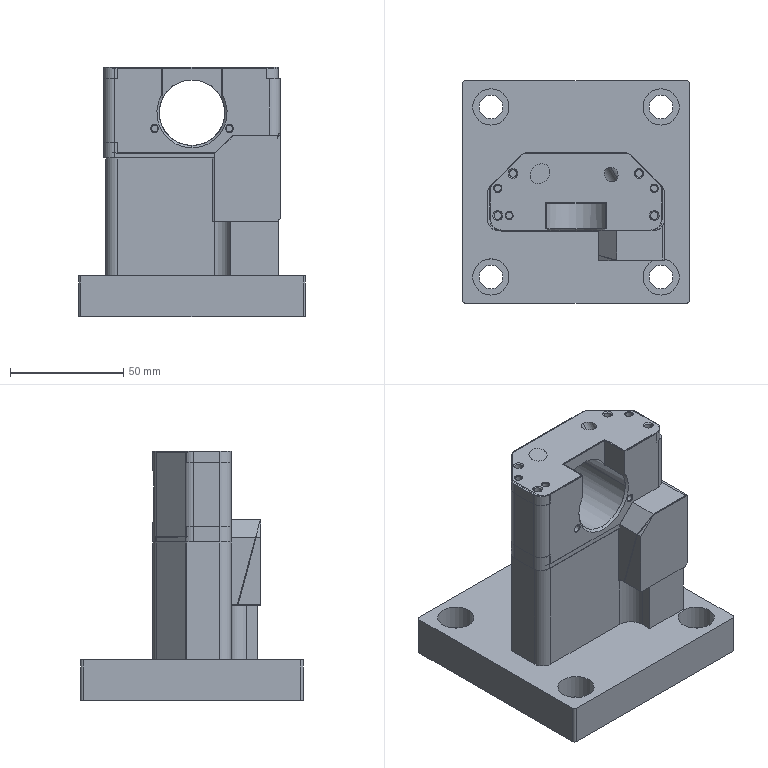NC program | NX | posted with a generic post | part box 100 x 98 x 110 mm
Lines 4432 to 5822 of 6635:
(HOLE_MILLING , TOOL : D4-12-D4-50-3T-ROUGH)
N8814 T03 M6
N8816 G54
N8818 G3P2 X0. Y0. Z0. I141. J33.2503 K72.627
N8820 G53.1
N8822 G17 G43 G0 G90 X29.203 Y-8.964 Z53.935 S4500 H3 M3
N8824 Z36.935
N8826 G94 G3 X29.793 Y-7.836 R0.9 F800.
N8828 X28.665 Y-7.246 R0.9
N8830 X28.665 Y-7.246 Z35.935 I0.537 J-1.718
N8832 X28.665 Y-7.246 Z34.935 I0.537 J-1.718
N8834 X28.665 Y-7.246 Z33.935 I0.537 J-1.718
N8836 X28.665 Y-7.246 Z32.935 I0.537 J-1.718
N8838 X28.665 Y-7.246 Z31.935 I0.537 J-1.718
N8840 X28.665 Y-7.246 Z30.935 I0.537 J-1.718
N8842 X28.665 Y-7.246 Z29.935 I0.537 J-1.718
N8844 X27.485 Y-9.501 R1.8
N8846 X28.665 Y-7.246 R-1.8
N8848 X28.075 Y-8.373 R0.9
N8850 X29.203 Y-8.964 R0.9
N8852 G0 Z53.935
N8854 G69
(HOLE_MILLING_COPY , TOOL : D4-12-D4-50-3T-ROUGH)
N8856 G3P2 X0. Y0. Z0. I-148. J25.2797 K77.0408
N8858 G53.1
N8860 X14.397 Y20.907 Z56.813 H3
N8862 Z39.813
N8864 G3 X14.697 Y21.386 R0.4
N8866 X14.218 Y21.686 R0.4
N8868 X14.218 Y21.686 Z38.813 I0.179 J-0.78
N8870 X14.218 Y21.686 Z37.813 I0.179 J-0.78
N8872 X14.218 Y21.686 Z36.813 I0.179 J-0.78
N8874 X14.218 Y21.686 Z35.813 I0.179 J-0.78
N8876 X14.218 Y21.686 Z34.813 I0.179 J-0.78
N8878 X14.218 Y21.686 Z33.813 I0.179 J-0.78
N8880 X14.218 Y21.686 Z32.813 I0.179 J-0.78
N8882 X14.218 Y21.686 Z31.813 I0.179 J-0.78
N8884 X13.618 Y20.727 R0.8
N8886 X14.218 Y21.686 R-0.8
N8888 X13.918 Y21.207 R0.4
N8890 X14.397 Y20.907 R0.4
N8892 G0 Z56.813
N8894 G69
N8896 M5
(SPOT_DRILLING_1 , TOOL : 点孔D6-65-90度)
N8898 T04 M6
N8900 G54
N8902 G17 G43 G0 G90 X-25.404 Y-23.388 B0. C314.959 S3000 H4 M3
N8904 Z60.
N8906 G94 G81 G98 Z38.2 F200. R43.
N8908 X-13.379 Y-28.329
N8910 X23.316 Y25.472
N8912 G80
(SPOT_DRILLING , TOOL : 点孔D6-65-90度)
N8914 G0 Z60.
N8916 X31.878 Y16.923
N8918 G81 Z38. F200. R43.
N8920 X13.983 Y25.324
N8922 X-25.304 Y-14.019
N8924 X-16.877 Y-31.903
N8926 G80
(SPOT_DRILLING_5 , TOOL : 点孔D6-65-90度)
N8928 G3P2 X0. Y0. Z0. I-148. J25.2797 K77.0408
N8930 G53.1
N8932 G0 X14.397 Y20.907 Z51.813 H4
N8934 G81 Z29.813 F200. R34.813
N8936 G80
N8938 G69
(SPOT_DRILLING_4 , TOOL : 点孔D6-65-90度)
N8940 G3P2 X0. Y0. Z0. I141. J33.2503 K72.627
N8942 G53.1
N8944 G0 X29.203 Y-8.964 Z49.935 H4
N8946 G81 Z26.435 F200. R32.935
N8948 G80
N8950 G69
(SPOT_DRILLING_3 , TOOL : 点孔D6-65-90度)
N8952 G19 G43 G0 Y37.25 Z13. B-180. C180. H4
N8954 X16.5
N8956 G17 G81 Y15.45 F200. R13.
N8958 X-16.5
N8960 G80
(SPOT_DRILLING_2 , TOOL : 点孔D6-65-90度)
N8962 G19 G43 G0 Y35.25 Z20. B-180. C0. H4
N8964 X17.5
N8966 G17 G81 Y12.45 F200. R20.
N8968 X-17.5
N8970 G80
N8972 M5
(SPOT_DRILLING_6 , TOOL : 钻头D8.0-81-114)
N8974 T05 M6
N8976 G54
N8978 G3P2 X0. Y0. Z0. I141. J33.2503 K-72.627
N8980 G53.1
N8982 G17 G43 G0 G90 X-18.887 Y24.009 Z49.935 S2000 H5 M3
N8984 G94 G83 G98 Z5.935 F200. Q3. R32.935
N8986 G80
N8988 G69
N8990 M5
(SPOT_DRILLING_7 , TOOL : 钻头D6.0-70-102)
N8992 T06 M6
N8994 G54
N8996 G3P2 X0. Y0. Z0. I-148. J25.2797 K-77.0408
N8998 G53.1
N9000 G17 G43 G0 G90 X-22.087 Y-12.511 Z51.813 S2000 H6 M3
N9002 G94 G83 G98 Z-11.187 F200. Q2.867 R34.813
N9004 G80
N9006 G69
N9008 M5
(SPOT_DRILLING_9 , TOOL : 钻头D2.8-39-67)
N9010 T08 M6
N9012 G54
N9014 G17 G0 G90 X12.626 Y32.139 B0. C109.041 S3000 M3
N9016 G43 Z60. H8
N9018 G94 G81 G98 Z32.8 F200. R43.
N9020 X-0.349 Y31.328
N9022 X-9.837 Y-33.102
N9024 G80
(SPOT_DRILLING_10 , TOOL : 钻头D2.8-39-67)
N9026 G19 G43 G0 Y37.25 Z13. B-180. C180. H8
N9028 X-16.5
N9030 G17 G81 Y10.05 F200. R13.
N9032 X16.5
N9034 G80
N9036 M5
(SPOT_DRILLING_11 , TOOL : 钻头D4.2-54-83)
N9038 T09 M6
N9040 G54
N9042 G19 G0 G90 Y35.25 Z20. B-180. C0. S3000 M3
N9044 G43 X-17.5 H9
N9046 G17 G94 G81 G98 Y7.95 F200. R20.
N9048 X17.5
N9050 G80
N9052 M5
(SPOT_DRILLING_8 , TOOL : 钻头D3.3-45-73)
N9054 T10 M6
N9056 G54
N9058 G17 G0 G90 X-27.8 Y8. B0. C0. S3000 M3
N9060 G43 Z60. H10
N9062 G94 G81 G98 Z30. F200. R43.
N9064 X-34.5 Y-10.6
N9066 X34.5
N9068 X27.8 Y8.
N9070 G80
N9072 M5
(SPOT_DRILLING_9_COPY , TOOL : D2.97插刀)
N9074 T11 M6
N9076 G54
N9078 G17 G0 G90 X-34.5 Y1.45 B0. C0. S3000 M3
N9080 G43 Z60. H11
N9082 G94 G81 G98 Z33. F60. R43.
N9084 X-29.5 Y-10.55
N9086 X34.5 Y1.5
N9088 G80
(SPOT_DRILLING_10_COPY , TOOL : D2.97插刀)
N9090 G19 G43 G0 Y37.25 Z13. B-180. C-180. H11
N9092 X-16.5
N9094 G17 G81 Y10.25 F60. R13.
N9096 X16.5
N9098 G80
N9100 M5
(THREAD_MILLING , TOOL : 螺纹铣刀M4-0.7)
N9102 T12 M6
N9104 G54
N9106 G17 G0 G90 X-34.5 Y10.6 B0. C-180. S4000 M3
N9108 G43 Z60. H12
N9110 Z31.325
N9112 G94 G3 X-34.598 Y10.723 Z31.5 I-0.049 J0.062 F100.
N9114 X-34.598 Y10.723 Z32.2 I0.098 J-0.123
N9116 X-34.5 Y10.6 Z32.375 I0.049 J-0.062
N9118 G0 Z33.425
N9120 G3 X-34.598 Y10.723 Z33.6 I-0.049 J0.062
N9122 X-34.598 Y10.723 Z34.3 I0.098 J-0.123
N9124 X-34.5 Y10.6 Z34.475 I0.049 J-0.062
N9126 G0 Z35.525
N9128 G3 X-34.598 Y10.723 Z35.7 I-0.049 J0.062
N9130 X-34.598 Y10.723 Z36.4 I0.098 J-0.123
N9132 X-34.5 Y10.6 Z36.575 I0.049 J-0.062
N9134 G0 Z37.625
N9136 G3 X-34.598 Y10.723 Z37.8 I-0.049 J0.062
N9138 X-34.598 Y10.723 Z38.5 I0.098 J-0.123
N9140 X-34.598 Y10.723 Z39.2 I0.098 J-0.123
N9142 X-34.358 Y10.532 Z39.6 R-0.157
N9144 X-34.5 Y10.6 Z39.775 I-0.071 J0.034
N9146 G0 Z31.325
N9148 G3 X-34.653 Y10.792 Z31.5 I-0.076 J0.096
N9150 X-34.653 Y10.792 Z32.2 I0.153 J-0.192
N9152 X-34.5 Y10.6 Z32.375 I0.076 J-0.096
N9154 G0 Z33.425
N9156 G3 X-34.653 Y10.792 Z33.6 I-0.076 J0.096
N9158 X-34.653 Y10.792 Z34.3 I0.153 J-0.192
N9160 X-34.5 Y10.6 Z34.475 I0.076 J-0.096
N9162 G0 Z35.525
N9164 G3 X-34.653 Y10.792 Z35.7 I-0.076 J0.096
N9166 X-34.653 Y10.792 Z36.4 I0.153 J-0.192
N9168 X-34.5 Y10.6 Z36.575 I0.076 J-0.096
N9170 G0 Z37.625
N9172 G3 X-34.653 Y10.792 Z37.8 I-0.076 J0.096
N9174 X-34.653 Y10.792 Z38.5 I0.153 J-0.192
N9176 X-34.653 Y10.792 Z39.2 I0.153 J-0.192
N9178 X-34.279 Y10.494 Z39.6 R-0.245
N9180 X-34.5 Y10.6 Z39.775 I-0.11 J0.053
N9182 G0 Z31.325
N9184 G3 X-34.707 Y10.86 Z31.5 I-0.104 J0.13
N9186 X-34.707 Y10.86 Z32.2 I0.207 J-0.26
N9188 X-34.5 Y10.6 Z32.375 I0.104 J-0.13
N9190 G0 Z33.425
N9192 G3 X-34.707 Y10.86 Z33.6 I-0.104 J0.13
N9194 X-34.707 Y10.86 Z34.3 I0.207 J-0.26
N9196 X-34.5 Y10.6 Z34.475 I0.104 J-0.13
N9198 G0 Z35.525
N9200 G3 X-34.707 Y10.86 Z35.7 I-0.104 J0.13
N9202 X-34.707 Y10.86 Z36.4 I0.207 J-0.26
N9204 X-34.5 Y10.6 Z36.575 I0.104 J-0.13
N9206 G0 Z37.625
N9208 G3 X-34.707 Y10.86 Z37.8 I-0.104 J0.13
N9210 X-34.707 Y10.86 Z38.5 I0.207 J-0.26
N9212 X-34.707 Y10.86 Z39.2 I0.207 J-0.26
N9214 X-34.2 Y10.456 Z39.6 R-0.332
N9216 X-34.5 Y10.6 Z39.775 I-0.15 J0.072
N9218 G0 Z31.325
N9220 G3 X-34.762 Y10.928 Z31.5 I-0.131 J0.164
N9222 X-34.762 Y10.928 Z32.2 I0.262 J-0.328
N9224 X-34.5 Y10.6 Z32.375 I0.131 J-0.164
N9226 G0 Z33.425
N9228 G3 X-34.762 Y10.928 Z33.6 I-0.131 J0.164
N9230 X-34.762 Y10.928 Z34.3 I0.262 J-0.328
N9232 X-34.5 Y10.6 Z34.475 I0.131 J-0.164
N9234 G0 Z35.525
N9236 G3 X-34.762 Y10.928 Z35.7 I-0.131 J0.164
N9238 X-34.762 Y10.928 Z36.4 I0.262 J-0.328
N9240 X-34.5 Y10.6 Z36.575 I0.131 J-0.164
N9242 G0 Z37.625
N9244 G3 X-34.762 Y10.928 Z37.8 I-0.131 J0.164
N9246 X-34.762 Y10.928 Z38.5 I0.262 J-0.328
N9248 X-34.762 Y10.928 Z39.2 I0.262 J-0.328
N9250 X-34.122 Y10.418 Z39.6 R-0.42
N9252 X-34.5 Y10.6 Z39.775 I-0.189 J0.091
N9254 G0 Z31.325
N9256 G3 X-34.762 Y10.928 Z31.5 I-0.131 J0.164
N9258 X-34.762 Y10.928 Z32.2 I0.262 J-0.328
N9260 X-34.5 Y10.6 Z32.375 I0.131 J-0.164
N9262 G0 Z33.425
N9264 G3 X-34.762 Y10.928 Z33.6 I-0.131 J0.164
N9266 X-34.762 Y10.928 Z34.3 I0.262 J-0.328
N9268 X-34.5 Y10.6 Z34.475 I0.131 J-0.164
N9270 G0 Z35.525
N9272 G3 X-34.762 Y10.928 Z35.7 I-0.131 J0.164
N9274 X-34.762 Y10.928 Z36.4 I0.262 J-0.328
N9276 X-34.5 Y10.6 Z36.575 I0.131 J-0.164
N9278 G0 Z37.625
N9280 G3 X-34.762 Y10.928 Z37.8 I-0.131 J0.164
N9282 X-34.762 Y10.928 Z38.5 I0.262 J-0.328
N9284 X-34.762 Y10.928 Z39.2 I0.262 J-0.328
N9286 X-34.122 Y10.418 Z39.6 R-0.42
N9288 X-34.5 Y10.6 Z39.775 I-0.189 J0.091
N9290 G0 Z31.325
N9292 G3 X-34.762 Y10.928 Z31.5 I-0.131 J0.164
N9294 X-34.762 Y10.928 Z32.2 I0.262 J-0.328
N9296 X-34.5 Y10.6 Z32.375 I0.131 J-0.164
N9298 G0 Z33.425
N9300 G3 X-34.762 Y10.928 Z33.6 I-0.131 J0.164
N9302 X-34.762 Y10.928 Z34.3 I0.262 J-0.328
N9304 X-34.5 Y10.6 Z34.475 I0.131 J-0.164
N9306 G0 Z35.525
N9308 G3 X-34.762 Y10.928 Z35.7 I-0.131 J0.164
N9310 X-34.762 Y10.928 Z36.4 I0.262 J-0.328
N9312 X-34.5 Y10.6 Z36.575 I0.131 J-0.164
N9314 G0 Z37.625
N9316 G3 X-34.762 Y10.928 Z37.8 I-0.131 J0.164
N9318 X-34.762 Y10.928 Z38.5 I0.262 J-0.328
N9320 X-34.762 Y10.928 Z39.2 I0.262 J-0.328
N9322 X-34.122 Y10.418 Z39.6 R-0.42
N9324 X-34.5 Y10.6 Z39.775 I-0.189 J0.091
N9326 G0 Z60.
N9328 X-27.8 Y-8.
N9330 Z31.325
N9332 G3 X-27.898 Y-7.877 Z31.5 I-0.049 J0.062
N9334 X-27.898 Y-7.877 Z32.2 I0.098 J-0.123
N9336 X-27.8 Y-8. Z32.375 I0.049 J-0.062
N9338 G0 Z33.425
N9340 G3 X-27.898 Y-7.877 Z33.6 I-0.049 J0.062
N9342 X-27.898 Y-7.877 Z34.3 I0.098 J-0.123
N9344 X-27.8 Y-8. Z34.475 I0.049 J-0.062
N9346 G0 Z35.525
N9348 G3 X-27.898 Y-7.877 Z35.7 I-0.049 J0.062
N9350 X-27.898 Y-7.877 Z36.4 I0.098 J-0.123
N9352 X-27.8 Y-8. Z36.575 I0.049 J-0.062
N9354 G0 Z37.625
N9356 G3 X-27.898 Y-7.877 Z37.8 I-0.049 J0.062
N9358 X-27.898 Y-7.877 Z38.5 I0.098 J-0.123
N9360 X-27.898 Y-7.877 Z39.2 I0.098 J-0.123
N9362 X-27.658 Y-8.068 Z39.6 R-0.157
N9364 X-27.8 Y-8. Z39.775 I-0.071 J0.034
N9366 G0 Z31.325
N9368 G3 X-27.953 Y-7.808 Z31.5 I-0.076 J0.096
N9370 X-27.953 Y-7.808 Z32.2 I0.153 J-0.192
N9372 X-27.8 Y-8. Z32.375 I0.076 J-0.096
N9374 G0 Z33.425
N9376 G3 X-27.953 Y-7.808 Z33.6 I-0.076 J0.096
N9378 X-27.953 Y-7.808 Z34.3 I0.153 J-0.192
N9380 X-27.8 Y-8. Z34.475 I0.076 J-0.096
N9382 G0 Z35.525
N9384 G3 X-27.953 Y-7.808 Z35.7 I-0.076 J0.096
N9386 X-27.953 Y-7.808 Z36.4 I0.153 J-0.192
N9388 X-27.8 Y-8. Z36.575 I0.076 J-0.096
N9390 G0 Z37.625
N9392 G3 X-27.953 Y-7.808 Z37.8 I-0.076 J0.096
N9394 X-27.953 Y-7.808 Z38.5 I0.153 J-0.192
N9396 X-27.953 Y-7.808 Z39.2 I0.153 J-0.192
N9398 X-27.579 Y-8.106 Z39.6 R-0.245
N9400 X-27.8 Y-8. Z39.775 I-0.11 J0.053
N9402 G0 Z31.325
N9404 G3 X-28.007 Y-7.74 Z31.5 I-0.104 J0.13
N9406 X-28.007 Y-7.74 Z32.2 I0.207 J-0.26
N9408 X-27.8 Y-8. Z32.375 I0.104 J-0.13
N9410 G0 Z33.425
N9412 G3 X-28.007 Y-7.74 Z33.6 I-0.104 J0.13
N9414 X-28.007 Y-7.74 Z34.3 I0.207 J-0.26
N9416 X-27.8 Y-8. Z34.475 I0.104 J-0.13
N9418 G0 Z35.525
N9420 G3 X-28.007 Y-7.74 Z35.7 I-0.104 J0.13
N9422 X-28.007 Y-7.74 Z36.4 I0.207 J-0.26
N9424 X-27.8 Y-8. Z36.575 I0.104 J-0.13
N9426 G0 Z37.625
N9428 G3 X-28.007 Y-7.74 Z37.8 I-0.104 J0.13
N9430 X-28.007 Y-7.74 Z38.5 I0.207 J-0.26
N9432 X-28.007 Y-7.74 Z39.2 I0.207 J-0.26
N9434 X-27.5 Y-8.144 Z39.6 R-0.332
N9436 X-27.8 Y-8. Z39.775 I-0.15 J0.072
N9438 G0 Z31.325
N9440 G3 X-28.062 Y-7.672 Z31.5 I-0.131 J0.164
N9442 X-28.062 Y-7.672 Z32.2 I0.262 J-0.328
N9444 X-27.8 Y-8. Z32.375 I0.131 J-0.164
N9446 G0 Z33.425
N9448 G3 X-28.062 Y-7.672 Z33.6 I-0.131 J0.164
N9450 X-28.062 Y-7.672 Z34.3 I0.262 J-0.328
N9452 X-27.8 Y-8. Z34.475 I0.131 J-0.164
N9454 G0 Z35.525
N9456 G3 X-28.062 Y-7.672 Z35.7 I-0.131 J0.164
N9458 X-28.062 Y-7.672 Z36.4 I0.262 J-0.328
N9460 X-27.8 Y-8. Z36.575 I0.131 J-0.164
N9462 G0 Z37.625
N9464 G3 X-28.062 Y-7.672 Z37.8 I-0.131 J0.164
N9466 X-28.062 Y-7.672 Z38.5 I0.262 J-0.328
N9468 X-28.062 Y-7.672 Z39.2 I0.262 J-0.328
N9470 X-27.422 Y-8.182 Z39.6 R-0.42
N9472 X-27.8 Y-8. Z39.775 I-0.189 J0.091
N9474 G0 Z31.325
N9476 G3 X-28.062 Y-7.672 Z31.5 I-0.131 J0.164
N9478 X-28.062 Y-7.672 Z32.2 I0.262 J-0.328
N9480 X-27.8 Y-8. Z32.375 I0.131 J-0.164
N9482 G0 Z33.425
N9484 G3 X-28.062 Y-7.672 Z33.6 I-0.131 J0.164
N9486 X-28.062 Y-7.672 Z34.3 I0.262 J-0.328
N9488 X-27.8 Y-8. Z34.475 I0.131 J-0.164
N9490 G0 Z35.525
N9492 G3 X-28.062 Y-7.672 Z35.7 I-0.131 J0.164
N9494 X-28.062 Y-7.672 Z36.4 I0.262 J-0.328
N9496 X-27.8 Y-8. Z36.575 I0.131 J-0.164
N9498 G0 Z37.625
N9500 G3 X-28.062 Y-7.672 Z37.8 I-0.131 J0.164
N9502 X-28.062 Y-7.672 Z38.5 I0.262 J-0.328
N9504 X-28.062 Y-7.672 Z39.2 I0.262 J-0.328
N9506 X-27.422 Y-8.182 Z39.6 R-0.42
N9508 X-27.8 Y-8. Z39.775 I-0.189 J0.091
N9510 G0 Z31.325
N9512 G3 X-28.062 Y-7.672 Z31.5 I-0.131 J0.164
N9514 X-28.062 Y-7.672 Z32.2 I0.262 J-0.328
N9516 X-27.8 Y-8. Z32.375 I0.131 J-0.164
N9518 G0 Z33.425
N9520 G3 X-28.062 Y-7.672 Z33.6 I-0.131 J0.164
N9522 X-28.062 Y-7.672 Z34.3 I0.262 J-0.328
N9524 X-27.8 Y-8. Z34.475 I0.131 J-0.164
N9526 G0 Z35.525
N9528 G3 X-28.062 Y-7.672 Z35.7 I-0.131 J0.164
N9530 X-28.062 Y-7.672 Z36.4 I0.262 J-0.328
N9532 X-27.8 Y-8. Z36.575 I0.131 J-0.164
N9534 G0 Z37.625
N9536 G3 X-28.062 Y-7.672 Z37.8 I-0.131 J0.164
N9538 X-28.062 Y-7.672 Z38.5 I0.262 J-0.328
N9540 X-28.062 Y-7.672 Z39.2 I0.262 J-0.328
N9542 X-27.422 Y-8.182 Z39.6 R-0.42
N9544 X-27.8 Y-8. Z39.775 I-0.189 J0.091
N9546 G0 Z60.
N9548 X27.8
N9550 Z31.325
N9552 G3 X27.702 Y-7.877 Z31.5 I-0.049 J0.062
N9554 X27.702 Y-7.877 Z32.2 I0.098 J-0.123
N9556 X27.8 Y-8. Z32.375 I0.049 J-0.062
N9558 G0 Z33.425
N9560 G3 X27.702 Y-7.877 Z33.6 I-0.049 J0.062
N9562 X27.702 Y-7.877 Z34.3 I0.098 J-0.123
N9564 X27.8 Y-8. Z34.475 I0.049 J-0.062
N9566 G0 Z35.525
N9568 G3 X27.702 Y-7.877 Z35.7 I-0.049 J0.062
N9570 X27.702 Y-7.877 Z36.4 I0.098 J-0.123
N9572 X27.8 Y-8. Z36.575 I0.049 J-0.062
N9574 G0 Z37.625
N9576 G3 X27.702 Y-7.877 Z37.8 I-0.049 J0.062
N9578 X27.702 Y-7.877 Z38.5 I0.098 J-0.123
N9580 X27.702 Y-7.877 Z39.2 I0.098 J-0.123
N9582 X27.942 Y-8.068 Z39.6 R-0.157
N9584 X27.8 Y-8. Z39.775 I-0.071 J0.034
N9586 G0 Z31.325
N9588 G3 X27.647 Y-7.808 Z31.5 I-0.076 J0.096
N9590 X27.647 Y-7.808 Z32.2 I0.153 J-0.192
N9592 X27.8 Y-8. Z32.375 I0.076 J-0.096
N9594 G0 Z33.425
N9596 G3 X27.647 Y-7.808 Z33.6 I-0.076 J0.096
N9598 X27.647 Y-7.808 Z34.3 I0.153 J-0.192
N9600 X27.8 Y-8. Z34.475 I0.076 J-0.096
N9602 G0 Z35.525
N9604 G3 X27.647 Y-7.808 Z35.7 I-0.076 J0.096
N9606 X27.647 Y-7.808 Z36.4 I0.153 J-0.192
N9608 X27.8 Y-8. Z36.575 I0.076 J-0.096
N9610 G0 Z37.625
N9612 G3 X27.647 Y-7.808 Z37.8 I-0.076 J0.096
N9614 X27.647 Y-7.808 Z38.5 I0.153 J-0.192
N9616 X27.647 Y-7.808 Z39.2 I0.153 J-0.192
N9618 X28.021 Y-8.106 Z39.6 R-0.245
N9620 X27.8 Y-8. Z39.775 I-0.11 J0.053
N9622 G0 Z31.325
N9624 G3 X27.593 Y-7.74 Z31.5 I-0.104 J0.13
N9626 X27.593 Y-7.74 Z32.2 I0.207 J-0.26
N9628 X27.8 Y-8. Z32.375 I0.104 J-0.13
N9630 G0 Z33.425
N9632 G3 X27.593 Y-7.74 Z33.6 I-0.104 J0.13
N9634 X27.593 Y-7.74 Z34.3 I0.207 J-0.26
N9636 X27.8 Y-8. Z34.475 I0.104 J-0.13
N9638 G0 Z35.525
N9640 G3 X27.593 Y-7.74 Z35.7 I-0.104 J0.13
N9642 X27.593 Y-7.74 Z36.4 I0.207 J-0.26
N9644 X27.8 Y-8. Z36.575 I0.104 J-0.13
N9646 G0 Z37.625
N9648 G3 X27.593 Y-7.74 Z37.8 I-0.104 J0.13
N9650 X27.593 Y-7.74 Z38.5 I0.207 J-0.26
N9652 X27.593 Y-7.74 Z39.2 I0.207 J-0.26
N9654 X28.1 Y-8.144 Z39.6 R-0.332
N9656 X27.8 Y-8. Z39.775 I-0.15 J0.072
N9658 G0 Z31.325
N9660 G3 X27.538 Y-7.672 Z31.5 I-0.131 J0.164
N9662 X27.538 Y-7.672 Z32.2 I0.262 J-0.328
N9664 X27.8 Y-8. Z32.375 I0.131 J-0.164
N9666 G0 Z33.425
N9668 G3 X27.538 Y-7.672 Z33.6 I-0.131 J0.164
N9670 X27.538 Y-7.672 Z34.3 I0.262 J-0.328
N9672 X27.8 Y-8. Z34.475 I0.131 J-0.164
N9674 G0 Z35.525
N9676 G3 X27.538 Y-7.672 Z35.7 I-0.131 J0.164
N9678 X27.538 Y-7.672 Z36.4 I0.262 J-0.328
N9680 X27.8 Y-8. Z36.575 I0.131 J-0.164
N9682 G0 Z37.625
N9684 G3 X27.538 Y-7.672 Z37.8 I-0.131 J0.164
N9686 X27.538 Y-7.672 Z38.5 I0.262 J-0.328
N9688 X27.538 Y-7.672 Z39.2 I0.262 J-0.328
N9690 X28.178 Y-8.182 Z39.6 R-0.42
N9692 X27.8 Y-8. Z39.775 I-0.189 J0.091
N9694 G0 Z31.325
N9696 G3 X27.538 Y-7.672 Z31.5 I-0.131 J0.164
N9698 X27.538 Y-7.672 Z32.2 I0.262 J-0.328
N9700 X27.8 Y-8. Z32.375 I0.131 J-0.164
N9702 G0 Z33.425
N9704 G3 X27.538 Y-7.672 Z33.6 I-0.131 J0.164
N9706 X27.538 Y-7.672 Z34.3 I0.262 J-0.328
N9708 X27.8 Y-8. Z34.475 I0.131 J-0.164
N9710 G0 Z35.525
N9712 G3 X27.538 Y-7.672 Z35.7 I-0.131 J0.164
N9714 X27.538 Y-7.672 Z36.4 I0.262 J-0.328
N9716 X27.8 Y-8. Z36.575 I0.131 J-0.164
N9718 G0 Z37.625
N9720 G3 X27.538 Y-7.672 Z37.8 I-0.131 J0.164
N9722 X27.538 Y-7.672 Z38.5 I0.262 J-0.328
N9724 X27.538 Y-7.672 Z39.2 I0.262 J-0.328
N9726 X28.178 Y-8.182 Z39.6 R-0.42
N9728 X27.8 Y-8. Z39.775 I-0.189 J0.091
N9730 G0 Z31.325
N9732 G3 X27.538 Y-7.672 Z31.5 I-0.131 J0.164
N9734 X27.538 Y-7.672 Z32.2 I0.262 J-0.328
N9736 X27.8 Y-8. Z32.375 I0.131 J-0.164
N9738 G0 Z33.425
N9740 G3 X27.538 Y-7.672 Z33.6 I-0.131 J0.164
N9742 X27.538 Y-7.672 Z34.3 I0.262 J-0.328
N9744 X27.8 Y-8. Z34.475 I0.131 J-0.164
N9746 G0 Z35.525
N9748 G3 X27.538 Y-7.672 Z35.7 I-0.131 J0.164
N9750 X27.538 Y-7.672 Z36.4 I0.262 J-0.328
N9752 X27.8 Y-8. Z36.575 I0.131 J-0.164
N9754 G0 Z37.625
N9756 G3 X27.538 Y-7.672 Z37.8 I-0.131 J0.164
N9758 X27.538 Y-7.672 Z38.5 I0.262 J-0.328
N9760 X27.538 Y-7.672 Z39.2 I0.262 J-0.328
N9762 X28.178 Y-8.182 Z39.6 R-0.42
N9764 X27.8 Y-8. Z39.775 I-0.189 J0.091
N9766 G0 Z60.
N9768 X34.5 Y10.6
N9770 Z31.325
N9772 G3 X34.402 Y10.723 Z31.5 I-0.049 J0.062
N9774 X34.402 Y10.723 Z32.2 I0.098 J-0.123
N9776 X34.5 Y10.6 Z32.375 I0.049 J-0.062
N9778 G0 Z33.425
N9780 G3 X34.402 Y10.723 Z33.6 I-0.049 J0.062
N9782 X34.402 Y10.723 Z34.3 I0.098 J-0.123
N9784 X34.5 Y10.6 Z34.475 I0.049 J-0.062
N9786 G0 Z35.525
N9788 G3 X34.402 Y10.723 Z35.7 I-0.049 J0.062
N9790 X34.402 Y10.723 Z36.4 I0.098 J-0.123
N9792 X34.5 Y10.6 Z36.575 I0.049 J-0.062
N9794 G0 Z37.625
N9796 G3 X34.402 Y10.723 Z37.8 I-0.049 J0.062
N9798 X34.402 Y10.723 Z38.5 I0.098 J-0.123
N9800 X34.402 Y10.723 Z39.2 I0.098 J-0.123
N9802 X34.642 Y10.532 Z39.6 R-0.157
N9804 X34.5 Y10.6 Z39.775 I-0.071 J0.034
N9806 G0 Z31.325
N9808 G3 X34.347 Y10.792 Z31.5 I-0.076 J0.096
N9810 X34.347 Y10.792 Z32.2 I0.153 J-0.192
N9812 X34.5 Y10.6 Z32.375 I0.076 J-0.096
N9814 G0 Z33.425
N9816 G3 X34.347 Y10.792 Z33.6 I-0.076 J0.096
N9818 X34.347 Y10.792 Z34.3 I0.153 J-0.192
N9820 X34.5 Y10.6 Z34.475 I0.076 J-0.096
N9822 G0 Z35.525
N9824 G3 X34.347 Y10.792 Z35.7 I-0.076 J0.096
N9826 X34.347 Y10.792 Z36.4 I0.153 J-0.192
N9828 X34.5 Y10.6 Z36.575 I0.076 J-0.096
N9830 G0 Z37.625
N9832 G3 X34.347 Y10.792 Z37.8 I-0.076 J0.096
N9834 X34.347 Y10.792 Z38.5 I0.153 J-0.192
N9836 X34.347 Y10.792 Z39.2 I0.153 J-0.192
N9838 X34.721 Y10.494 Z39.6 R-0.245
N9840 X34.5 Y10.6 Z39.775 I-0.11 J0.053
N9842 G0 Z31.325
N9844 G3 X34.293 Y10.86 Z31.5 I-0.104 J0.13
N9846 X34.293 Y10.86 Z32.2 I0.207 J-0.26
N9848 X34.5 Y10.6 Z32.375 I0.104 J-0.13
N9850 G0 Z33.425
N9852 G3 X34.293 Y10.86 Z33.6 I-0.104 J0.13
N9854 X34.293 Y10.86 Z34.3 I0.207 J-0.26
N9856 X34.5 Y10.6 Z34.475 I0.104 J-0.13
N9858 G0 Z35.525
N9860 G3 X34.293 Y10.86 Z35.7 I-0.104 J0.13
N9862 X34.293 Y10.86 Z36.4 I0.207 J-0.26
N9864 X34.5 Y10.6 Z36.575 I0.104 J-0.13
N9866 G0 Z37.625
N9868 G3 X34.293 Y10.86 Z37.8 I-0.104 J0.13
N9870 X34.293 Y10.86 Z38.5 I0.207 J-0.26
N9872 X34.293 Y10.86 Z39.2 I0.207 J-0.26
N9874 X34.8 Y10.456 Z39.6 R-0.332
N9876 X34.5 Y10.6 Z39.775 I-0.15 J0.072
N9878 G0 Z31.325
N9880 G3 X34.238 Y10.928 Z31.5 I-0.131 J0.164
N9882 X34.238 Y10.928 Z32.2 I0.262 J-0.328
N9884 X34.5 Y10.6 Z32.375 I0.131 J-0.164
N9886 G0 Z33.425
N9888 G3 X34.238 Y10.928 Z33.6 I-0.131 J0.164
N9890 X34.238 Y10.928 Z34.3 I0.262 J-0.328
N9892 X34.5 Y10.6 Z34.475 I0.131 J-0.164
N9894 G0 Z35.525
N9896 G3 X34.238 Y10.928 Z35.7 I-0.131 J0.164
N9898 X34.238 Y10.928 Z36.4 I0.262 J-0.328
N9900 X34.5 Y10.6 Z36.575 I0.131 J-0.164
N9902 G0 Z37.625
N9904 G3 X34.238 Y10.928 Z37.8 I-0.131 J0.164
N9906 X34.238 Y10.928 Z38.5 I0.262 J-0.328
N9908 X34.238 Y10.928 Z39.2 I0.262 J-0.328
N9910 X34.878 Y10.418 Z39.6 R-0.42
N9912 X34.5 Y10.6 Z39.775 I-0.189 J0.091
N9914 G0 Z31.325
N9916 G3 X34.238 Y10.928 Z31.5 I-0.131 J0.164
N9918 X34.238 Y10.928 Z32.2 I0.262 J-0.328
N9920 X34.5 Y10.6 Z32.375 I0.131 J-0.164
N9922 G0 Z33.425
N9924 G3 X34.238 Y10.928 Z33.6 I-0.131 J0.164
N9926 X34.238 Y10.928 Z34.3 I0.262 J-0.328
N9928 X34.5 Y10.6 Z34.475 I0.131 J-0.164
N9930 G0 Z35.525
N9932 G3 X34.238 Y10.928 Z35.7 I-0.131 J0.164
N9934 X34.238 Y10.928 Z36.4 I0.262 J-0.328
N9936 X34.5 Y10.6 Z36.575 I0.131 J-0.164
N9938 G0 Z37.625
N9940 G3 X34.238 Y10.928 Z37.8 I-0.131 J0.164
N9942 X34.238 Y10.928 Z38.5 I0.262 J-0.328
N9944 X34.238 Y10.928 Z39.2 I0.262 J-0.328
N9946 X34.878 Y10.418 Z39.6 R-0.42
N9948 X34.5 Y10.6 Z39.775 I-0.189 J0.091
N9950 G0 Z31.325
N9952 G3 X34.238 Y10.928 Z31.5 I-0.131 J0.164
N9954 X34.238 Y10.928 Z32.2 I0.262 J-0.328
N9956 X34.5 Y10.6 Z32.375 I0.131 J-0.164
N9958 G0 Z33.425
N9960 G3 X34.238 Y10.928 Z33.6 I-0.131 J0.164
N9962 X34.238 Y10.928 Z34.3 I0.262 J-0.328
N9964 X34.5 Y10.6 Z34.475 I0.131 J-0.164
N9966 G0 Z35.525
N9968 G3 X34.238 Y10.928 Z35.7 I-0.131 J0.164
N9970 X34.238 Y10.928 Z36.4 I0.262 J-0.328
N9972 X34.5 Y10.6 Z36.575 I0.131 J-0.164
N9974 G0 Z37.625
N9976 G3 X34.238 Y10.928 Z37.8 I-0.131 J0.164
N9978 X34.238 Y10.928 Z38.5 I0.262 J-0.328
N9980 X34.238 Y10.928 Z39.2 I0.262 J-0.328
N9982 X34.878 Y10.418 Z39.6 R-0.42
N9984 X34.5 Y10.6 Z39.775 I-0.189 J0.091
N9986 G0 Z60.
(THREAD_MILLING_1 , TOOL : 螺纹铣刀M4-0.7)
N9988 G19 G43 Y35.25 Z20. B-180. C0. H12
N9990 X-17.5
N9992 G17 Y7.579
N9994 G1 X-17.481 Z19.994
N9996 G18 G3 X-17.635 Y7.75 Z19.408 R0.303
N9998 X-17.635 Y8.45 Z19.408 I0.135 K0.592
N10000 X-17.52 Y8.621 Z20.003 R0.303
N10002 G17 G1 X-17.5 Z20.
N10004 G0 Y9.679
N10006 G1 X-17.481 Z19.994
N10008 G18 G3 X-17.635 Y9.85 Z19.408 R0.303
N10010 X-17.635 Y10.55 Z19.408 I0.135 K0.592
N10012 X-17.52 Y10.721 Z20.003 R0.303
N10014 G17 G1 X-17.5 Z20.
N10016 G0 Y11.779
N10018 G1 X-17.481 Z19.994
N10020 G18 G3 X-17.635 Y11.95 Z19.408 R0.303
N10022 X-17.635 Y12.65 Z19.408 I0.135 K0.592
N10024 X-17.52 Y12.821 Z20.003 R0.303
N10026 G17 G1 X-17.5 Z20.
N10028 G0 Y13.879
N10030 G1 X-17.481 Z19.994
N10032 G18 G3 X-17.635 Y14.05 Z19.408 R0.303
N10034 X-17.635 Y14.75 Z19.408 I0.135 K0.592
N10036 X-18.047 Y14.85 Z19.736 R0.608
N10038 X-17.51 Y15.021 Z20.017 R0.303
N10040 G17 G1 X-17.5 Z20.
N10042 G0 Y7.578
N10044 G1 X-17.481 Z19.994
N10046 G18 G3 X-17.655 Y7.75 Z19.322 R0.347
N10048 X-17.655 Y8.45 Z19.322 I0.155 K0.678
N10050 X-17.52 Y8.622 Z20.003 R0.347
N10052 G17 G1 X-17.5 Z20.
N10054 G0 Y9.678
N10056 G1 X-17.481 Z19.994
N10058 G18 G3 X-17.655 Y9.85 Z19.322 R0.347
N10060 X-17.655 Y10.55 Z19.322 I0.155 K0.678
N10062 X-17.52 Y10.722 Z20.003 R0.347
N10064 G17 G1 X-17.5 Z20.
N10066 G0 Y11.778
N10068 G1 X-17.481 Z19.994
N10070 G18 G3 X-17.655 Y11.95 Z19.322 R0.347
N10072 X-17.655 Y12.65 Z19.322 I0.155 K0.678
N10074 X-17.52 Y12.822 Z20.003 R0.347
N10076 G17 G1 X-17.5 Z20.
N10078 G0 Y13.878
N10080 G1 X-17.481 Z19.994
N10082 G18 G3 X-17.655 Y14.05 Z19.322 R0.347
N10084 X-17.655 Y14.75 Z19.322 I0.155 K0.678
N10086 X-18.126 Y14.85 Z19.698 R0.695
N10088 X-17.51 Y15.022 Z20.017 R0.347
N10090 G17 G1 X-17.5 Z20.
N10092 G0 Y7.578
N10094 G1 X-17.481 Z19.995
N10096 G18 G3 X-17.674 Y7.75 Z19.237 R0.391
N10098 X-17.674 Y8.45 Z19.237 I0.174 K0.763
N10100 X-17.52 Y8.622 Z20.003 R0.391
N10102 G17 G1 X-17.5 Z20.
N10104 G0 Y9.678
N10106 G1 X-17.481 Z19.995
N10108 G18 G3 X-17.674 Y9.85 Z19.237 R0.391
N10110 X-17.674 Y10.55 Z19.237 I0.174 K0.763
N10112 X-17.52 Y10.722 Z20.003 R0.391
N10114 G17 G1 X-17.5 Z20.
N10116 G0 Y11.778
N10118 G1 X-17.481 Z19.995
N10120 G18 G3 X-17.674 Y11.95 Z19.237 R0.391
N10122 X-17.674 Y12.65 Z19.237 I0.174 K0.763
N10124 X-17.52 Y12.822 Z20.003 R0.391
N10126 G17 G1 X-17.5 Z20.
N10128 G0 Y13.878
N10130 G1 X-17.481 Z19.995
N10132 G18 G3 X-17.674 Y14.05 Z19.237 R0.391
N10134 X-17.674 Y14.75 Z19.237 I0.174 K0.763
N10136 X-18.205 Y14.85 Z19.66 R0.783
N10138 X-17.51 Y15.022 Z20.018 R0.391
N10140 G17 G1 X-17.5 Z20.
N10142 G0 Y7.578
N10144 G1 X-17.481 Z19.995
N10146 G18 G3 X-17.694 Y7.75 Z19.152 R0.435
N10148 X-17.694 Y8.45 Z19.152 I0.194 K0.848
N10150 X-17.52 Y8.622 Z20.004 R0.435
N10152 G17 G1 X-17.5 Z20.
N10154 G0 Y9.678
N10156 G1 X-17.481 Z19.995
N10158 G18 G3 X-17.694 Y9.85 Z19.152 R0.435
N10160 X-17.694 Y10.55 Z19.152 I0.194 K0.848
N10162 X-17.52 Y10.722 Z20.004 R0.435
N10164 G17 G1 X-17.5 Z20.
N10166 G0 Y11.778
N10168 G1 X-17.481 Z19.995
N10170 G18 G3 X-17.694 Y11.95 Z19.152 R0.435
N10172 X-17.694 Y12.65 Z19.152 I0.194 K0.848
N10174 X-17.52 Y12.822 Z20.004 R0.435
N10176 G17 G1 X-17.5 Z20.
N10178 G0 Y13.878
N10180 G1 X-17.481 Z19.995
N10182 G18 G3 X-17.694 Y14.05 Z19.152 R0.435
N10184 X-17.694 Y14.75 Z19.152 I0.194 K0.848
N10186 X-18.284 Y14.85 Z19.623 R0.87
N10188 X-17.509 Y15.022 Z20.018 R0.435
N10190 G17 G1 X-17.5 Z20.
N10192 G0 Y7.578
N10194 G1 X-17.481 Z19.995
N10196 G18 G3 X-17.694 Y7.75 Z19.152 R0.435
N10198 X-17.694 Y8.45 Z19.152 I0.194 K0.848
N10200 X-17.52 Y8.622 Z20.004 R0.435
N10202 G17 G1 X-17.5 Z20.
N10204 G0 Y9.678
N10206 G1 X-17.481 Z19.995
N10208 G18 G3 X-17.694 Y9.85 Z19.152 R0.435
N10210 X-17.694 Y10.55 Z19.152 I0.194 K0.848
N10212 X-17.52 Y10.722 Z20.004 R0.435
N10214 G17 G1 X-17.5 Z20.
N10216 G0 Y11.778
N10218 G1 X-17.481 Z19.995
N10220 G18 G3 X-17.694 Y11.95 Z19.152 R0.435
N10222 X-17.694 Y12.65 Z19.152 I0.194 K0.848
N10224 X-17.52 Y12.822 Z20.004 R0.435
N10226 G17 G1 X-17.5 Z20.
N10228 G0 Y13.878
N10230 G1 X-17.481 Z19.995
N10232 G18 G3 X-17.694 Y14.05 Z19.152 R0.435
N10234 X-17.694 Y14.75 Z19.152 I0.194 K0.848
N10236 X-18.284 Y14.85 Z19.623 R0.87
N10238 X-17.509 Y15.022 Z20.018 R0.435
N10240 G17 G1 X-17.5 Z20.
N10242 G0 Y7.578
N10244 G1 X-17.481 Z19.995
N10246 G18 G3 X-17.694 Y7.75 Z19.152 R0.435
N10248 X-17.694 Y8.45 Z19.152 I0.194 K0.848
N10250 X-17.52 Y8.622 Z20.004 R0.435
N10252 G17 G1 X-17.5 Z20.
N10254 G0 Y9.678
N10256 G1 X-17.481 Z19.995
N10258 G18 G3 X-17.694 Y9.85 Z19.152 R0.435
N10260 X-17.694 Y10.55 Z19.152 I0.194 K0.848
N10262 X-17.52 Y10.722 Z20.004 R0.435
N10264 G17 G1 X-17.5 Z20.
N10266 G0 Y11.778
N10268 G1 X-17.481 Z19.995
N10270 G18 G3 X-17.694 Y11.95 Z19.152 R0.435
N10272 X-17.694 Y12.65 Z19.152 I0.194 K0.848
N10274 X-17.52 Y12.822 Z20.004 R0.435
N10276 G17 G1 X-17.5 Z20.
N10278 G0 Y13.878
N10280 G1 X-17.481 Z19.995
N10282 G18 G3 X-17.694 Y14.05 Z19.152 R0.435
N10284 X-17.694 Y14.75 Z19.152 I0.194 K0.848
N10286 X-18.284 Y14.85 Z19.623 R0.87
N10288 X-17.509 Y15.022 Z20.018 R0.435
N10290 G17 G1 X-17.5 Z20.
N10292 G0 Y35.25
N10294 X17.5
N10296 Y7.579
N10298 G1 X17.519 Z19.994
N10300 G18 G3 X17.365 Y7.75 Z19.408 R0.303
N10302 X17.365 Y8.45 Z19.408 I0.135 K0.592
N10304 X17.48 Y8.621 Z20.003 R0.303
N10306 G17 G1 X17.5 Z20.
N10308 G0 Y9.679
N10310 G1 X17.519 Z19.994
N10312 G18 G3 X17.365 Y9.85 Z19.408 R0.303
N10314 X17.365 Y10.55 Z19.408 I0.135 K0.592
N10316 X17.48 Y10.721 Z20.003 R0.303
N10318 G17 G1 X17.5 Z20.
N10320 G0 Y11.779
N10322 G1 X17.519 Z19.994
N10324 G18 G3 X17.365 Y11.95 Z19.408 R0.303
N10326 X17.365 Y12.65 Z19.408 I0.135 K0.592
N10328 X17.48 Y12.821 Z20.003 R0.303
N10330 G17 G1 X17.5 Z20.
N10332 G0 Y13.879
N10334 G1 X17.519 Z19.994
N10336 G18 G3 X17.365 Y14.05 Z19.408 R0.303
N10338 X17.365 Y14.75 Z19.408 I0.135 K0.592
N10340 X16.953 Y14.85 Z19.736 R0.607
N10342 X17.49 Y15.021 Z20.017 R0.303
N10344 G17 G1 X17.5 Z20.
N10346 G0 Y7.578
N10348 G1 X17.519 Z19.994
N10350 G18 G3 X17.345 Y7.75 Z19.322 R0.347
N10352 X17.345 Y8.45 Z19.322 I0.155 K0.678
N10354 X17.48 Y8.622 Z20.003 R0.347
N10356 G17 G1 X17.5 Z20.
N10358 G0 Y9.678
N10360 G1 X17.519 Z19.994
N10362 G18 G3 X17.345 Y9.85 Z19.322 R0.347
N10364 X17.345 Y10.55 Z19.322 I0.155 K0.678
N10366 X17.48 Y10.722 Z20.003 R0.347
N10368 G17 G1 X17.5 Z20.
N10370 G0 Y11.778
N10372 G1 X17.519 Z19.994
N10374 G18 G3 X17.345 Y11.95 Z19.322 R0.347
N10376 X17.345 Y12.65 Z19.322 I0.155 K0.678
N10378 X17.48 Y12.822 Z20.003 R0.347
N10380 G17 G1 X17.5 Z20.
N10382 G0 Y13.878
N10384 G1 X17.519 Z19.994
N10386 G18 G3 X17.345 Y14.05 Z19.322 R0.347
N10388 X17.345 Y14.75 Z19.322 I0.155 K0.678
N10390 X16.874 Y14.85 Z19.698 R0.695
N10392 X17.49 Y15.022 Z20.017 R0.347
N10394 G17 G1 X17.5 Z20.
N10396 G0 Y7.578
N10398 G1 X17.519 Z19.995
N10400 G18 G3 X17.326 Y7.75 Z19.237 R0.391
N10402 X17.326 Y8.45 Z19.237 I0.174 K0.763
N10404 X17.48 Y8.622 Z20.003 R0.391
N10406 G17 G1 X17.5 Z20.
N10408 G0 Y9.678
N10410 G1 X17.519 Z19.995
N10412 G18 G3 X17.326 Y9.85 Z19.237 R0.391
N10414 X17.326 Y10.55 Z19.237 I0.174 K0.763
N10416 X17.48 Y10.722 Z20.003 R0.391
N10418 G17 G1 X17.5 Z20.
N10420 G0 Y11.778
N10422 G1 X17.519 Z19.995
N10424 G18 G3 X17.326 Y11.95 Z19.237 R0.391
N10426 X17.326 Y12.65 Z19.237 I0.174 K0.763
N10428 X17.48 Y12.822 Z20.003 R0.391
N10430 G17 G1 X17.5 Z20.
N10432 G0 Y13.878
N10434 G1 X17.519 Z19.995
N10436 G18 G3 X17.326 Y14.05 Z19.237 R0.391
N10438 X17.326 Y14.75 Z19.237 I0.174 K0.763
N10440 X16.795 Y14.85 Z19.66 R0.783
N10442 X17.49 Y15.022 Z20.018 R0.391
N10444 G17 G1 X17.5 Z20.
N10446 G0 Y7.578
N10448 G1 X17.519 Z19.995
N10450 G18 G3 X17.306 Y7.75 Z19.152 R0.435
N10452 X17.306 Y8.45 Z19.152 I0.194 K0.848
N10454 X17.48 Y8.622 Z20.004 R0.435
N10456 G17 G1 X17.5 Z20.
N10458 G0 Y9.678
N10460 G1 X17.519 Z19.995
N10462 G18 G3 X17.306 Y9.85 Z19.152 R0.435
N10464 X17.306 Y10.55 Z19.152 I0.194 K0.848
N10466 X17.48 Y10.722 Z20.004 R0.435
N10468 G17 G1 X17.5 Z20.
N10470 G0 Y11.778
N10472 G1 X17.519 Z19.995
N10474 G18 G3 X17.306 Y11.95 Z19.152 R0.435
N10476 X17.306 Y12.65 Z19.152 I0.194 K0.848
N10478 X17.48 Y12.822 Z20.004 R0.435
N10480 G17 G1 X17.5 Z20.
N10482 G0 Y13.878
N10484 G1 X17.519 Z19.995
N10486 G18 G3 X17.306 Y14.05 Z19.152 R0.435
N10488 X17.306 Y14.75 Z19.152 I0.194 K0.848
N10490 X16.716 Y14.85 Z19.623 R0.87
N10492 X17.491 Y15.022 Z20.018 R0.435
N10494 G17 G1 X17.5 Z20.
N10496 G0 Y7.578
N10498 G1 X17.519 Z19.995
N10500 G18 G3 X17.306 Y7.75 Z19.152 R0.435
N10502 X17.306 Y8.45 Z19.152 I0.194 K0.848
N10504 X17.48 Y8.622 Z20.004 R0.435
N10506 G17 G1 X17.5 Z20.
N10508 G0 Y9.678
N10510 G1 X17.519 Z19.995
N10512 G18 G3 X17.306 Y9.85 Z19.152 R0.435
N10514 X17.306 Y10.55 Z19.152 I0.194 K0.848
N10516 X17.48 Y10.722 Z20.004 R0.435
N10518 G17 G1 X17.5 Z20.
N10520 G0 Y11.778
N10522 G1 X17.519 Z19.995
N10524 G18 G3 X17.306 Y11.95 Z19.152 R0.435
N10526 X17.306 Y12.65 Z19.152 I0.194 K0.848
N10528 X17.48 Y12.822 Z20.004 R0.435
N10530 G17 G1 X17.5 Z20.
N10532 G0 Y13.878
N10534 G1 X17.519 Z19.995
N10536 G18 G3 X17.306 Y14.05 Z19.152 R0.435
N10538 X17.306 Y14.75 Z19.152 I0.194 K0.848
N10540 X16.716 Y14.85 Z19.623 R0.87
N10542 X17.491 Y15.022 Z20.018 R0.435
N10544 G17 G1 X17.5 Z20.
N10546 G0 Y7.578
N10548 G1 X17.519 Z19.995
N10550 G18 G3 X17.306 Y7.75 Z19.152 R0.435
N10552 X17.306 Y8.45 Z19.152 I0.194 K0.848
N10554 X17.48 Y8.622 Z20.004 R0.435
N10556 G17 G1 X17.5 Z20.
N10558 G0 Y9.678
N10560 G1 X17.519 Z19.995
N10562 G18 G3 X17.306 Y9.85 Z19.152 R0.435
N10564 X17.306 Y10.55 Z19.152 I0.194 K0.848
N10566 X17.48 Y10.722 Z20.004 R0.435
N10568 G17 G1 X17.5 Z20.
N10570 G0 Y11.778
N10572 G1 X17.519 Z19.995
N10574 G18 G3 X17.306 Y11.95 Z19.152 R0.435
N10576 X17.306 Y12.65 Z19.152 I0.194 K0.848
N10578 X17.48 Y12.822 Z20.004 R0.435
N10580 G17 G1 X17.5 Z20.
N10582 G0 Y13.878
N10584 G1 X17.519 Z19.995
N10586 G18 G3 X17.306 Y14.05 Z19.152 R0.435
N10588 X17.306 Y14.75 Z19.152 I0.194 K0.848
N10590 X16.716 Y14.85 Z19.623 R0.87
N10592 X17.491 Y15.022 Z20.018 R0.435
N10594 G17 G1 X17.5 Z20.
N10596 G0 Y35.25
N10598 M5
(PLANAR_MILL_7 , TOOL : D16-48-D16-100-3T-FINISH)
N10600 T14 M6
N10602 G54
N10604 G17 G0 G90 X48. Y4.279 B0. C0. S4500 M3
N10606 G43 Z60. H14
N10608 Z36.9
N10610 G94 G1 Z34.9 F800.
N10612 G3 X46. Y2.279 R2.
N10614 G1 Y-12.25
N10616 G2 X33. Y-25.25 R13.
N10618 G3 X31. Y-27.25 R2.
N10620 G1 Z36.9
N10622 G0 Z60.
N10624 X-31.
N10626 Z36.9
N10628 G1 Z34.9
N10630 G3 X-33. Y-25.25 R2.
N10632 G2 X-46. Y-12.25 R13.
N10634 G1 Y2.279
N10636 G3 X-48. Y4.279 R2.
N10638 G1 Z36.9
N10640 G0 Z60.
(PLANAR_MILL_6_COPY , TOOL : D16-48-D16-100-3T-FINISH)
N10642 X-31. Y-27.25
N10644 Z1.
N10646 G1 Z-1.
N10648 G3 X-33. Y-25.25 R2.
N10650 G1 X-34.
N10652 G2 X-47. Y-12.25 R13.
N10654 G1 Y-0.721
N10656 G2 X-43.192 Y8.471 R13.
N10658 G1 X-30.221 Y21.442
N10660 G2 X-21.029 Y25.25 R13.
N10662 G1 X21.029
N10664 G2 X30.221 Y21.442 R13.
N10666 G1 X43.192 Y8.471
N10668 G2 X47. Y-0.721 R13.
N10670 G1 Y-14.721
N10672 G3 X49. Y-16.721 R2.
N10674 G1 Z1.
N10676 G0 Z60.
N10678 X-31. Y-27.25
N10680 Z1.
N10682 G1 Z-1.
N10684 G3 X-33. Y-25.25 R2.
N10686 G1 X-34.
N10688 G2 X-47. Y-12.25 R13.
N10690 G1 Y-0.721
N10692 G2 X-43.192 Y8.471 R13.
N10694 G1 X-30.221 Y21.442
N10696 G2 X-21.029 Y25.25 R13.
N10698 G1 X21.029
N10700 G2 X30.221 Y21.442 R13.
N10702 G1 X43.192 Y8.471
N10704 G2 X47. Y-0.721 R13.
N10706 G1 Y-14.721
N10708 G3 X49. Y-16.721 R2.
N10710 G1 Z1.
N10712 G0 Z60.
(PLANAR_MILL_6_COPY_COPY , TOOL : D16-48-D16-100-3T-FINISH)
N10714 X44.8 Y9.879
N10716 Z55.
N10718 Z12.01
N10720 G1 Z10.01
N10722 G3 X44.4 Y7.079 R2.
N10724 G2 X47. Y-0.721 R13.
N10726 G1 Y-12.25
N10728 G2 X34. Y-25.25 R13.
N10730 G3 X32. Y-27.25 R2.
N10732 G1 Z12.01
N10734 G0 Z55.
N10736 X44.8 Y9.879
N10738 Z12.01
N10740 G1 Z10.01
N10742 G3 X44.4 Y7.079 R2.
N10744 G2 X47. Y-0.721 R13.
N10746 G1 Y-12.25
N10748 G2 X34. Y-25.25 R13.
N10750 G3 X32. Y-27.25 R2.
N10752 G1 Z12.01
N10754 G0 Z55.
(PLANAR_MILL_8 , TOOL : D16-48-D16-100-3T-FINISH)
N10756 G19 G43 Y37.25 Z20.4 B-180. C0. H14
N10758 X-4.5
N10760 Y17.25
N10762 G1 Y15.25
N10764 G18 G3 X-12.5 Y15.25 Z28.4 R8.
N10766 G19 G1 X12.5
N10768 G18 G3 X14.4 Y15.25 Z26.5 R1.9
N10770 G19 G1 Z13.5
N10772 G18 G3 X12.5 Y15.25 Z11.6 R1.9
N10774 G19 G1 X-12.5
N10776 G18 G3 X-14.4 Y15.25 Z13.5 R1.9
N10778 G19 G1 Z26.5
N10780 G18 G3 X-12.5 Y15.25 Z28.4 R1.9
N10782 X-4.5 Y15.25 Z20.4 R8.
N10784 G19 G1 Y17.25
N10786 G0 Y37.25
(PLANAR_MILL_8_COPY , TOOL : D16-48-D16-100-3T-FINISH)
N10788 Z20.5
N10790 Y17.26
N10792 G1 Y15.26
N10794 G18 G3 X-12.5 Y15.26 Z28.5 R8.
N10796 G19 G1 X12.5
N10798 G18 G3 X14.5 Y15.26 Z26.5 R2.
N10800 G19 G1 Z13.5
N10802 G18 G3 X12.5 Y15.26 Z11.5 R2.
N10804 G19 G1 X-12.5
N10806 G18 G3 X-14.5 Y15.26 Z13.5 R2.
N10808 G19 G1 Z26.5
N10810 G18 G3 X-12.5 Y15.26 Z28.5 R2.
N10812 X-4.5 Y15.26 Z20.5 R8.
N10814 G19 G1 Y17.26
N10816 G0 Y37.25
(PLANAR_MILL_3_COPY , TOOL : D16-48-D16-100-3T-FINISH)
N10818 G43 Y37.25 Z55.7 B-180. C-180. H14
N10820 X4.9
N10822 Y8.1
N10824 G1 Y5.1
N10826 Z39.7
N10828 Z26.423
N10830 G18 G2 X5.738 Y5.1 Z22.835 R8.1
N10832 G3 X-5.738 Y5.1 Z22.835 R-6.4
N10834 G2 X-4.9 Y5.1 Z26.423 R8.1
N10836 G19 G1 Z39.7
N10838 Z55.7
N10840 Y8.1
N10842 G0 Y37.25
(PLANAR_MILL_12 , TOOL : D16-48-D16-100-3T-FINISH)
N10844 X5.
N10846 Y37.25 Z49.7
N10848 Y7.05
N10850 G1 Y5.05
N10852 Z39.7
N10854 Z26.423
N10856 Z16.423
N10858 Y7.05
N10860 G0 Y37.25
N10862 X-5.
N10864 Y7.05
N10866 G1 Y5.05
N10868 Z26.423
N10870 Z39.7
N10872 Z49.7
N10874 Y7.05
N10876 G0 Y37.25
(PLANAR_MILL_3_COPY_COPY , TOOL : D16-48-D16-100-3T-FINISH)
N10878 X4.9
N10880 Y37.25 Z55.7
N10882 Y8.06
N10884 G1 Y5.06
N10886 Z39.7
N10888 Z26.423
N10890 G18 G2 X5.738 Y5.06 Z22.835 R8.1
N10892 G3 X-5.738 Y5.06 Z22.835 R-6.4
N10894 G2 X-4.9 Y5.06 Z26.423 R8.1
N10896 G19 G1 Z39.7
N10898 Z55.7
N10900 Y8.06
N10902 G0 Y37.25
(PLANAR_MILL_2_COPY , TOOL : D16-48-D16-100-3T-FINISH)
N10904 X-2.
N10906 Y42.25 Z-43.7
N10908 Y20.21
N10910 G1 Y17.21
N10912 Z-27.7
N10914 Z2.
N10916 G18 G2 X-4.343 Y17.21 Z7.657 R8.
N10918 G19 G1 X-12.334 Z15.647
N10920 G18 G2 X-17.987 Y17.21 Z17.99 R8.
N10922 G19 G1 X-37.986 Z18.
N10924 X-53.986 Z18.008
N10926 Y20.21
N10928 G0 Y42.25
(PLANAR_MILL_4_COPY , TOOL : D16-48-D16-100-3T-FINISH)
N10930 X10.757
N10932 Y37.25 Z55.7
N10934 Y20.21
N10936 G1 Y17.21
N10938 Z39.7
N10940 X-33.
N10942 Z35.
N10944 X-34.
N10946 Z18.1
N10948 X-18.
N10950 G18 G3 X-12.272 Y17.21 Z15.728 R8.1
N10952 G19 G1 X1.155 Z2.3
N10954 X33.
N10956 Z7.
N10958 X34.
N10960 Z35.
N10962 X33.
N10964 Z39.7
N10966 X10.757
N10968 Z30.1
N10970 X-24.4
N10972 Z27.7
N10974 X-18.
N10976 G18 G3 X-5.484 Y17.21 Z22.516 R17.7
N10978 G19 G1 X5.132 Z11.9
N10980 X24.4
N10982 Z30.1
N10984 X10.757
N10986 Z22.9
N10988 X4.314
N10990 X8.114 Z19.1
N10992 X17.2
N10994 Z22.9
N10996 X10.757
N10998 Z55.7
N11000 Y20.21
N11002 G0 Y37.25
(PLANAR_MILL_22 , TOOL : D16-48-D16-100-3T-FINISH)
N11004 G43 Y58. Z-21. B-180. C-90. S5500 H14
N11006 X-14.75
N11008 Y40.
N11010 G1 Y38. F600.
N11012 X-4.75
N11014 X32.721
N11016 X42.721
N11018 Y40.
N11020 G0 Y58.
N11022 X-14.75 Z-9.
N11024 Y40.
N11026 G1 Y38.
N11028 X-4.75
N11030 X32.721
N11032 X42.721
N11034 Y40.
N11036 G0 Y58.
N11038 X-14.75 Z2.125
N11040 Y40.
N11042 G1 Y38.
N11044 X-4.75 Z3.
N11046 X32.721
N11048 X34.721
N11050 Y40.
N11052 G0 Y58.
N11054 M5
(PLANAR_MILL_9 , TOOL : 点孔D8-79-90度)
N11056 T15 M6
N11058 G54
N11060 G19 G0 G90 Y37.25 Z44.031 B-180. C-180. S3500 M3
N11062 G43 X14.926 H15
N11064 Y17.25
N11066 G94 G1 Y15.25 F1000.
N11068 X12.098 Z41.202
N11070 X11.886 Z40.99
N11072 G18 G2 X11.3 Y15.25 Z39.576 R2.
N11074 G19 G1 Z27.877
N11076 Z23.877
N11078 Y17.25
N11080 G0 Y37.25
N11082 X-11.3
N11084 Y17.25
N11086 G1 Y15.25
N11088 Z27.877
N11090 Z39.576
N11092 G18 G2 X-11.886 Y15.25 Z40.99 R2.
N11094 G19 G1 X-12.098 Z41.202
N11096 X-14.926 Z44.031
N11098 Y17.25
N11100 G0 Y37.25
(PLANAR_MILL_9_COPY , TOOL : 点孔D8-79-90度)
N11102 X10.332
N11104 Y37.25 Z29.566
N11106 Y17.25
N11108 G1 Y15.25
N11110 X12.103 Z25.98
N11112 G18 G3 X-12.103 Y15.25 Z25.98 R-13.5
N11114 G19 G1 X-10.332 Z29.566
N11116 Y17.25
N11118 G0 Y37.25
(PLANAR_MILL_10 , TOOL : 点孔D8-79-90度)
N11120 G17 G43 X41.7 Y-0.226 B0. C-180. H15
N11122 Z60.
N11124 Z40.
N11126 G1 Z38.
N11128 G3 X39.7 Y-2.226 R2.
N11130 G2 X39.114 Y-3.64 R2.
N11132 G1 X25.767 Y-16.988
N11134 G2 X21.029 Y-18.95 R6.7
N11136 G1 X-21.029
N11138 G2 X-25.767 Y-16.988 R6.7
N11140 G1 X-38.738 Y-4.017
N11142 G2 X-39.274 Y-3.411 R6.7
N11144 X-39.7 Y-2.177 R2.
N11146 G1 Y12.25
N11148 G2 X-33. Y18.95 R6.7
N11150 G1 X-13.424
N11152 G2 X-12.01 Y18.364 R2.
N11154 G1 X-11.886 Y18.24
N11156 G2 X-11.3 Y16.826 R2.
N11158 G1 Y6.75
N11160 X11.3
N11162 Y16.826
N11164 G2 X11.886 Y18.24 R2.
N11166 G1 X12.01 Y18.364
N11168 G2 X13.424 Y18.95 R2.
N11170 G1 X33.
N11172 G2 X39.7 Y12.25 R6.7
N11174 G1 Y-2.226
N11176 G3 X41.7 Y-4.226 R2.
N11178 G1 Z40.
N11180 G0 Z60.
(PLANAR_MILL_10_COPY , TOOL : 点孔D8-79-90度)
N11182 G19 G43 Y37.25 Z7.001 B-180. C0. H15
N11184 X14.5
N11186 Y17.75
N11188 G1 Y15.75
N11190 Z6.7
N11192 G18 G3 X12.5 Y15.75 Z4.7 R2.
N11194 G19 G1 X-12.5
N11196 G18 G3 X-19.77 Y15.75 Z8.542 R8.8
N11198 X-21.3 Y15.75 Z13.499 R8.803
N11200 G19 G1 Z26.497
N11202 G18 G3 X-19.772 Y15.75 Z31.455 R8.805
N11204 X-12.5 Y15.75 Z35.3 R8.8
N11206 G19 G1 X12.5
N11208 G18 G3 X19.77 Y15.75 Z31.458 R8.8
N11210 X21.3 Y15.75 Z26.502 R8.794
N11212 G19 G1 Z13.503
N11214 G18 G3 X19.772 Y15.75 Z8.545 R8.805
N11216 X12.5 Y15.75 Z4.7 R8.8
N11218 X10.5 Y15.75 Z6.7 R2.
N11220 G19 G1 Y17.75
N11222 G0 Y37.25
(PLANAR_MILL_10_COPY_COPY , TOOL : 点孔D8-79-90度)
N11224 Y35.25 Z10.508
N11226 X2.
N11228 Y14.25
N11230 G1 Y12.25
N11232 Z10.3
N11234 G18 G3 X0. Y12.25 Z8.3 R2.
N11236 X-11.7 Y12.25 Z20. R11.7
N11238 X0. Y12.25 Z8.3 R-11.7
N11240 X-2. Y12.25 Z10.3 R2.
N11242 G19 G1 Z10.508
N11244 Y14.25
N11246 G0 Y35.25
(CURVE_DRIVE , TOOL : 点孔D8-79-90度)
N11248 G17 G43 X12.646 Y-20.95 B0. C0. S4000 H15
N11250 Z60.
N11252 Z43.346
N11254 G1 Y-20.85 Z42.456 F600.
N11256 Y-20.554 Z41.611
N11258 Y-20.077 Z40.852
N11260 Y-19.444 Z40.219
N11262 Y-18.686 Z39.743
N11264 Y-17.84 Z39.447
N11266 Y-16.95 Z39.346
N11268 Y-5.404
N11270 X13.004 Y-5.046 Z39.704
N11272 X13.147 Y-4.903 Z39.847
N11274 X13.3 Y-4.75 Z40.
N11276 X13.269 Y-4.781 Z39.969
N11278 X13.259 Y-4.791 Z39.959
N11280 X13.239 Y-4.811 Z39.939
N11282 X13.218 Y-4.832 Z39.918
N11284 X13.167 Y-4.883 Z39.867
N11286 X13.004 Y-5.046 Z39.704
N11288 X12.646 Y-5.404 Z39.346
N11290 X-12.646
N11292 X-8.121 Z43.872
N11294 G0 X-13.976 Y-4.074 Z45.575
N11296 G1 X-14.282 Y-3.768 Z44.791
N11298 X-14.456 Y-3.594 Z43.93
N11300 X-14.491 Y-3.559 Z43.035
N11302 X-14.384 Y-3.666 Z42.152
N11304 X-14.14 Y-3.91 Z41.325
N11306 X-13.773 Y-4.277 Z40.596
N11308 X-13.3 Y-4.75 Z40.
N11310 X-13.004 Y-5.046 Z39.704
N11312 X-12.646 Y-5.404 Z39.346
N11314 Y-16.95
N11316 Y-17.84 Z39.447
N11318 Y-18.686 Z39.743
N11320 Y-19.444 Z40.219
N11322 Y-20.077 Z40.852
N11324 Y-20.554 Z41.611
N11326 Y-20.85 Z42.456
N11328 Y-20.95 Z43.346
N11330 G0 Z60.
N11332 M5
(PLANAR_MILL_21 , TOOL : D50面刀)
N11334 T01 M6
N11336 G54
N11338 G17 G0 G90 X68.971 Y-3.05 B0. C0. S4000 M3
N11340 G43 Z60. H1
N11342 Z41.95
N11344 G94 G1 Z39.95 F600.
N11346 X38.971
N11348 X-38.971
N11350 X-68.971
N11352 Z41.95
N11354 G0 Z60.
(PLANAR_MILL_21_COPY , TOOL : D50面刀)
N11356 X68.971
N11358 Z41.905
N11360 G1 Z39.905
N11362 X38.971
N11364 X-38.971
N11366 X-68.971
N11368 Z41.905
N11370 G0 Z60.
N11372 M5